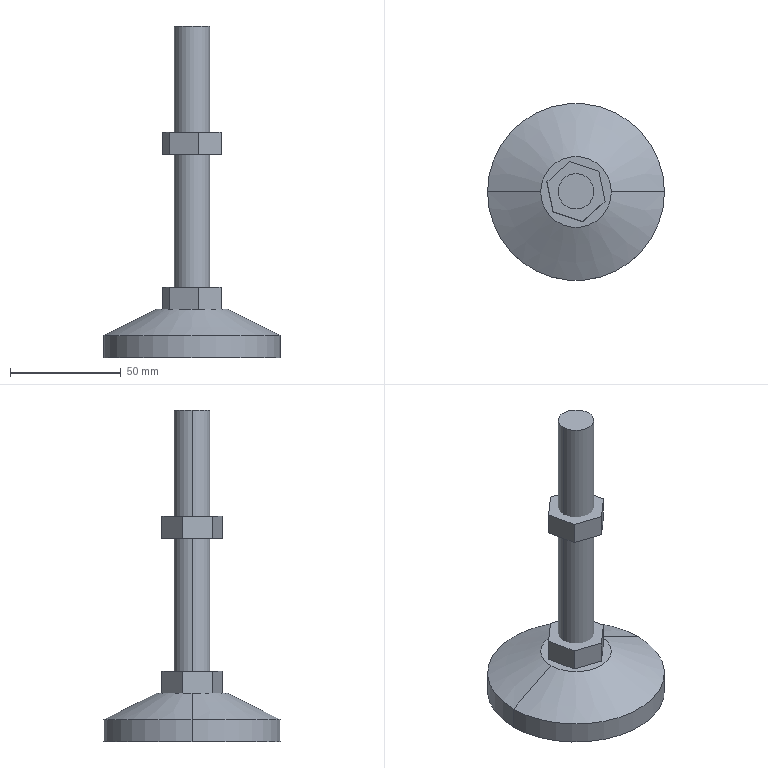Part | SolidWorks | features BaseBody 3 | 3 solids | 37 faces | box 80 x 80 x 150 mm | volume 92663 mm3 | plane 27 | cylinder 6 | torus 2 | cone 2 | commonest cylinder face diameters 16 x2 30 x2 80 x2
STEP:
#1=CARTESIAN_POINT('',(8.,0.,150.));
#2=VERTEX_POINT('',#1);
#3=CARTESIAN_POINT('',(-8.,0.,150.));
#4=VERTEX_POINT('',#3);
#5=CARTESIAN_POINT('',(0.,0.,150.));
#6=DIRECTION('',(0.,0.,1.));
#7=DIRECTION('',(1.,0.,0.));
#8=AXIS2_PLACEMENT_3D('',#5,#6,#7);
#9=CIRCLE('',#8,8.);
#10=EDGE_CURVE('',#2,#4,#9,.T.);
#11=ORIENTED_EDGE('',*,*,#10,.F.);
#12=CARTESIAN_POINT('',(8.,0.,22.));
#13=VERTEX_POINT('',#12);
#14=CARTESIAN_POINT('',(8.,0.,150.));
#15=DIRECTION('',(0.,0.,-1.));
#16=VECTOR('',#15,1000.);
#17=LINE('',#14,#16);
#18=EDGE_CURVE('',#2,#13,#17,.T.);
#19=ORIENTED_EDGE('',*,*,#18,.T.);
#20=CARTESIAN_POINT('',(-8.,0.,22.));
#21=VERTEX_POINT('',#20);
#22=CARTESIAN_POINT('',(0.,0.,22.));
#23=DIRECTION('',(0.,0.,1.));
#24=DIRECTION('',(-1.,0.,0.));
#25=AXIS2_PLACEMENT_3D('',#22,#23,#24);
#26=CIRCLE('',#25,8.);
#27=EDGE_CURVE('',#13,#21,#26,.T.);
#28=ORIENTED_EDGE('',*,*,#27,.T.);
#29=CARTESIAN_POINT('',(-8.,0.,150.));
#30=DIRECTION('',(0.,0.,-1.));
#31=VECTOR('',#30,1000.);
#32=LINE('',#29,#31);
#33=EDGE_CURVE('',#4,#21,#32,.T.);
#34=ORIENTED_EDGE('',*,*,#33,.F.);
#35=EDGE_LOOP('',(#11,#19,#28,#34));
#36=FACE_OUTER_BOUND('',#35,.T.);
#37=CARTESIAN_POINT('',(0.,0.,150.));
#38=DIRECTION('',(0.,0.,-1.));
#39=DIRECTION('',(-1.,0.,0.));
#40=AXIS2_PLACEMENT_3D('',#37,#38,#39);
#41=CYLINDRICAL_SURFACE('',#40,8.);
#42=ADVANCED_FACE('',(#36),#41,.T.);
#43=CARTESIAN_POINT('',(0.,-15.,13.));
#44=VERTEX_POINT('',#43);
#45=CARTESIAN_POINT('',(0.,15.,13.));
#46=VERTEX_POINT('',#45);
#47=CARTESIAN_POINT('',(0.,0.,13.));
#48=DIRECTION('',(0.,0.,-1.));
#49=DIRECTION('',(0.,1.,0.));
#50=AXIS2_PLACEMENT_3D('',#47,#48,#49);
#51=CIRCLE('',#50,15.);
#52=EDGE_CURVE('',#44,#46,#51,.T.);
#53=ORIENTED_EDGE('',*,*,#52,.F.);
#54=CARTESIAN_POINT('',(0.,-15.,12.));
#55=VERTEX_POINT('',#54);
#56=CARTESIAN_POINT('',(0.,-15.,13.));
#57=DIRECTION('',(0.,0.,-1.));
#58=VECTOR('',#57,1000.);
#59=LINE('',#56,#58);
#60=EDGE_CURVE('',#44,#55,#59,.T.);
#61=ORIENTED_EDGE('',*,*,#60,.T.);
#62=CARTESIAN_POINT('',(0.,15.,12.));
#63=VERTEX_POINT('',#62);
#64=CARTESIAN_POINT('',(0.,0.,12.));
#65=DIRECTION('',(0.,0.,-1.));
#66=DIRECTION('',(0.,1.,0.));
#67=AXIS2_PLACEMENT_3D('',#64,#65,#66);
#68=CIRCLE('',#67,15.);
#69=EDGE_CURVE('',#55,#63,#68,.T.);
#70=ORIENTED_EDGE('',*,*,#69,.T.);
#71=CARTESIAN_POINT('',(0.,15.,13.));
#72=DIRECTION('',(0.,0.,-1.));
#73=VECTOR('',#72,1000.);
#74=LINE('',#71,#73);
#75=EDGE_CURVE('',#46,#63,#74,.T.);
#76=ORIENTED_EDGE('',*,*,#75,.F.);
#77=EDGE_LOOP('',(#53,#61,#70,#76));
#78=FACE_OUTER_BOUND('',#77,.T.);
#79=CARTESIAN_POINT('',(0.,0.,13.));
#80=DIRECTION('',(0.,0.,-1.));
#81=DIRECTION('',(0.,1.,0.));
#82=AXIS2_PLACEMENT_3D('',#79,#80,#81);
#83=CYLINDRICAL_SURFACE('',#82,15.);
#84=ADVANCED_FACE('',(#78),#83,.F.);
#85=ORIENTED_EDGE('',*,*,#69,.F.);
#86=CARTESIAN_POINT('',(0.,-34.,0.));
#87=VERTEX_POINT('',#86);
#88=CARTESIAN_POINT('',(0.,-9.731,-17.385));
#89=DIRECTION('',(1.,0.,0.));
#90=DIRECTION('',(0.,1.,0.));
#91=AXIS2_PLACEMENT_3D('',#88,#89,#90);
#92=CIRCLE('',#91,29.854);
#93=EDGE_CURVE('',#55,#87,#92,.T.);
#94=ORIENTED_EDGE('',*,*,#93,.T.);
#95=CARTESIAN_POINT('',(0.,34.,0.));
#96=VERTEX_POINT('',#95);
#97=CARTESIAN_POINT('',(0.,0.,0.));
#98=DIRECTION('',(0.,0.,-1.));
#99=DIRECTION('',(0.,1.,0.));
#100=AXIS2_PLACEMENT_3D('',#97,#98,#99);
#101=CIRCLE('',#100,34.);
#102=EDGE_CURVE('',#87,#96,#101,.T.);
#103=ORIENTED_EDGE('',*,*,#102,.T.);
#104=CARTESIAN_POINT('',(0.,9.731,-17.385));
#105=DIRECTION('',(-1.,0.,0.));
#106=DIRECTION('',(0.,0.,1.));
#107=AXIS2_PLACEMENT_3D('',#104,#105,#106);
#108=CIRCLE('',#107,29.854);
#109=EDGE_CURVE('',#63,#96,#108,.T.);
#110=ORIENTED_EDGE('',*,*,#109,.F.);
#111=EDGE_LOOP('',(#85,#94,#103,#110));
#112=FACE_OUTER_BOUND('',#111,.T.);
#113=CARTESIAN_POINT('',(0.,0.,-17.385));
#114=DIRECTION('',(0.,0.,-1.));
#115=DIRECTION('',(0.,1.,0.));
#116=AXIS2_PLACEMENT_3D('',#113,#114,#115);
#117=TOROIDAL_SURFACE('',#116,9.731,29.854);
#118=ADVANCED_FACE('',(#112),#117,.F.);
#119=CARTESIAN_POINT('',(-16.,0.,22.));
#120=VERTEX_POINT('',#119);
#121=CARTESIAN_POINT('',(16.,0.,22.));
#122=VERTEX_POINT('',#121);
#123=CARTESIAN_POINT('',(0.,0.,22.));
#124=DIRECTION('',(0.,0.,-1.));
#125=DIRECTION('',(-1.,0.,0.));
#126=AXIS2_PLACEMENT_3D('',#123,#124,#125);
#127=CIRCLE('',#126,16.);
#128=EDGE_CURVE('',#120,#122,#127,.T.);
#129=ORIENTED_EDGE('',*,*,#128,.T.);
#130=CARTESIAN_POINT('',(40.,0.,10.));
#131=VERTEX_POINT('',#130);
#132=CARTESIAN_POINT('',(16.,0.,22.));
#133=DIRECTION('',(0.8944,0.,-0.4472));
#134=VECTOR('',#133,1000.);
#135=LINE('',#132,#134);
#136=EDGE_CURVE('',#122,#131,#135,.T.);
#137=ORIENTED_EDGE('',*,*,#136,.T.);
#138=CARTESIAN_POINT('',(-40.,0.,10.));
#139=VERTEX_POINT('',#138);
#140=CARTESIAN_POINT('',(0.,0.,10.));
#141=DIRECTION('',(0.,0.,1.));
#142=DIRECTION('',(1.,0.,0.));
#143=AXIS2_PLACEMENT_3D('',#140,#141,#142);
#144=CIRCLE('',#143,40.);
#145=EDGE_CURVE('',#131,#139,#144,.T.);
#146=ORIENTED_EDGE('',*,*,#145,.T.);
#147=CARTESIAN_POINT('',(-16.,0.,22.));
#148=DIRECTION('',(-0.8944,0.,-0.4472));
#149=VECTOR('',#148,1000.);
#150=LINE('',#147,#149);
#151=EDGE_CURVE('',#120,#139,#150,.T.);
#152=ORIENTED_EDGE('',*,*,#151,.F.);
#153=EDGE_LOOP('',(#129,#137,#146,#152));
#154=FACE_OUTER_BOUND('',#153,.T.);
#155=CARTESIAN_POINT('',(0.,0.,22.));
#156=DIRECTION('',(0.,0.,-1.));
#157=DIRECTION('',(-1.,0.,0.));
#158=AXIS2_PLACEMENT_3D('',#155,#156,#157);
#159=CONICAL_SURFACE('',#158,16.,1.107);
#160=ADVANCED_FACE('',(#154),#159,.T.);
#161=ORIENTED_EDGE('',*,*,#145,.F.);
#162=CARTESIAN_POINT('',(40.,0.,0.));
#163=VERTEX_POINT('',#162);
#164=CARTESIAN_POINT('',(40.,0.,10.));
#165=DIRECTION('',(0.,0.,-1.));
#166=VECTOR('',#165,1000.);
#167=LINE('',#164,#166);
#168=EDGE_CURVE('',#131,#163,#167,.T.);
#169=ORIENTED_EDGE('',*,*,#168,.T.);
#170=CARTESIAN_POINT('',(-40.,0.,0.));
#171=VERTEX_POINT('',#170);
#172=CARTESIAN_POINT('',(0.,0.,0.));
#173=DIRECTION('',(0.,0.,1.));
#174=DIRECTION('',(1.,0.,0.));
#175=AXIS2_PLACEMENT_3D('',#172,#173,#174);
#176=CIRCLE('',#175,40.);
#177=EDGE_CURVE('',#163,#171,#176,.T.);
#178=ORIENTED_EDGE('',*,*,#177,.T.);
#179=CARTESIAN_POINT('',(-40.,0.,10.));
#180=DIRECTION('',(0.,0.,-1.));
#181=VECTOR('',#180,1000.);
#182=LINE('',#179,#181);
#183=EDGE_CURVE('',#139,#171,#182,.T.);
#184=ORIENTED_EDGE('',*,*,#183,.F.);
#185=EDGE_LOOP('',(#161,#169,#178,#184));
#186=FACE_OUTER_BOUND('',#185,.T.);
#187=CARTESIAN_POINT('',(0.,0.,10.));
#188=DIRECTION('',(0.,0.,-1.));
#189=DIRECTION('',(-1.,0.,0.));
#190=AXIS2_PLACEMENT_3D('',#187,#188,#189);
#191=CYLINDRICAL_SURFACE('',#190,40.);
#192=ADVANCED_FACE('',(#186),#191,.T.);
#193=ORIENTED_EDGE('',*,*,#128,.F.);
#194=CARTESIAN_POINT('',(0.,0.,22.));
#195=DIRECTION('',(0.,0.,-1.));
#196=DIRECTION('',(-1.,0.,0.));
#197=AXIS2_PLACEMENT_3D('',#194,#195,#196);
#198=CIRCLE('',#197,16.);
#199=EDGE_CURVE('',#122,#120,#198,.T.);
#200=ORIENTED_EDGE('',*,*,#199,.F.);
#201=EDGE_LOOP('',(#193,#200));
#202=FACE_OUTER_BOUND('',#201,.T.);
#203=CARTESIAN_POINT('',(0.,0.,22.));
#204=DIRECTION('',(0.,0.,1.));
#205=DIRECTION('',(-1.,0.,0.));
#206=AXIS2_PLACEMENT_3D('',#203,#204,#205);
#207=CIRCLE('',#206,8.);
#208=EDGE_CURVE('',#21,#13,#207,.T.);
#209=ORIENTED_EDGE('',*,*,#208,.F.);
#210=ORIENTED_EDGE('',*,*,#27,.F.);
#211=EDGE_LOOP('',(#209,#210));
#212=FACE_BOUND('',#211,.T.);
#213=CARTESIAN_POINT('',(0.,0.,22.));
#214=DIRECTION('',(0.,0.,-1.));
#215=DIRECTION('',(-1.,0.,0.));
#216=AXIS2_PLACEMENT_3D('',#213,#214,#215);
#217=PLANE('',#216);
#218=ADVANCED_FACE('',(#202,#212),#217,.F.);
#219=CARTESIAN_POINT('',(0.,0.,13.));
#220=DIRECTION('',(0.,0.,-1.));
#221=DIRECTION('',(0.,1.,0.));
#222=AXIS2_PLACEMENT_3D('',#219,#220,#221);
#223=CIRCLE('',#222,15.);
#224=EDGE_CURVE('',#46,#44,#223,.T.);
#225=ORIENTED_EDGE('',*,*,#224,.T.);
#226=ORIENTED_EDGE('',*,*,#52,.T.);
#227=EDGE_LOOP('',(#225,#226));
#228=FACE_OUTER_BOUND('',#227,.T.);
#229=CARTESIAN_POINT('',(-11.89,7.115,13.));
#230=VERTEX_POINT('',#229);
#231=CARTESIAN_POINT('',(0.2164,13.855,13.));
#232=VERTEX_POINT('',#231);
#233=CARTESIAN_POINT('',(-11.89,7.115,13.));
#234=DIRECTION('',(0.8737,0.4864,0.));
#235=VECTOR('',#234,1000.);
#236=LINE('',#233,#235);
#237=EDGE_CURVE('',#230,#232,#236,.T.);
#238=ORIENTED_EDGE('',*,*,#237,.F.);
#239=CARTESIAN_POINT('',(-12.107,-6.74,13.));
#240=VERTEX_POINT('',#239);
#241=CARTESIAN_POINT('',(-12.107,-6.74,13.));
#242=DIRECTION('',(0.01561,0.9999,0.));
#243=VECTOR('',#242,1000.);
#244=LINE('',#241,#243);
#245=EDGE_CURVE('',#240,#230,#244,.T.);
#246=ORIENTED_EDGE('',*,*,#245,.F.);
#247=CARTESIAN_POINT('',(-0.2164,-13.855,13.));
#248=VERTEX_POINT('',#247);
#249=CARTESIAN_POINT('',(-0.2164,-13.855,13.));
#250=DIRECTION('',(-0.8581,0.5135,0.));
#251=VECTOR('',#250,1000.);
#252=LINE('',#249,#251);
#253=EDGE_CURVE('',#248,#240,#252,.T.);
#254=ORIENTED_EDGE('',*,*,#253,.F.);
#255=CARTESIAN_POINT('',(11.89,-7.115,13.));
#256=VERTEX_POINT('',#255);
#257=CARTESIAN_POINT('',(11.89,-7.115,13.));
#258=DIRECTION('',(-0.8737,-0.4864,0.));
#259=VECTOR('',#258,1000.);
#260=LINE('',#257,#259);
#261=EDGE_CURVE('',#256,#248,#260,.T.);
#262=ORIENTED_EDGE('',*,*,#261,.F.);
#263=CARTESIAN_POINT('',(12.107,6.74,13.));
#264=VERTEX_POINT('',#263);
#265=CARTESIAN_POINT('',(12.107,6.74,13.));
#266=DIRECTION('',(-0.01561,-0.9999,0.));
#267=VECTOR('',#266,1000.);
#268=LINE('',#265,#267);
#269=EDGE_CURVE('',#264,#256,#268,.T.);
#270=ORIENTED_EDGE('',*,*,#269,.F.);
#271=CARTESIAN_POINT('',(0.2164,13.855,13.));
#272=DIRECTION('',(0.8581,-0.5135,0.));
#273=VECTOR('',#272,1000.);
#274=LINE('',#271,#273);
#275=EDGE_CURVE('',#232,#264,#274,.T.);
#276=ORIENTED_EDGE('',*,*,#275,.F.);
#277=EDGE_LOOP('',(#238,#246,#254,#262,#270,#276));
#278=FACE_BOUND('',#277,.T.);
#279=CARTESIAN_POINT('',(0.,0.,13.));
#280=DIRECTION('',(0.,0.,-1.));
#281=DIRECTION('',(0.,1.,0.));
#282=AXIS2_PLACEMENT_3D('',#279,#280,#281);
#283=PLANE('',#282);
#284=ADVANCED_FACE('',(#228,#278),#283,.T.);
#285=ORIENTED_EDGE('',*,*,#168,.F.);
#286=CARTESIAN_POINT('',(0.,0.,10.));
#287=DIRECTION('',(0.,0.,1.));
#288=DIRECTION('',(1.,0.,0.));
#289=AXIS2_PLACEMENT_3D('',#286,#287,#288);
#290=CIRCLE('',#289,40.);
#291=EDGE_CURVE('',#139,#131,#290,.T.);
#292=ORIENTED_EDGE('',*,*,#291,.F.);
#293=ORIENTED_EDGE('',*,*,#183,.T.);
#294=CARTESIAN_POINT('',(0.,0.,0.));
#295=DIRECTION('',(0.,0.,1.));
#296=DIRECTION('',(1.,0.,0.));
#297=AXIS2_PLACEMENT_3D('',#294,#295,#296);
#298=CIRCLE('',#297,40.);
#299=EDGE_CURVE('',#171,#163,#298,.T.);
#300=ORIENTED_EDGE('',*,*,#299,.T.);
#301=EDGE_LOOP('',(#285,#292,#293,#300));
#302=FACE_OUTER_BOUND('',#301,.T.);
#303=CARTESIAN_POINT('',(0.,0.,10.));
#304=DIRECTION('',(0.,0.,-1.));
#305=DIRECTION('',(-1.,0.,0.));
#306=AXIS2_PLACEMENT_3D('',#303,#304,#305);
#307=CYLINDRICAL_SURFACE('',#306,40.);
#308=ADVANCED_FACE('',(#302),#307,.T.);
#309=CARTESIAN_POINT('',(0.,0.,0.));
#310=DIRECTION('',(0.,0.,-1.));
#311=DIRECTION('',(0.,1.,0.));
#312=AXIS2_PLACEMENT_3D('',#309,#310,#311);
#313=CIRCLE('',#312,34.);
#314=EDGE_CURVE('',#96,#87,#313,.T.);
#315=ORIENTED_EDGE('',*,*,#314,.F.);
#316=ORIENTED_EDGE('',*,*,#102,.F.);
#317=EDGE_LOOP('',(#315,#316));
#318=FACE_BOUND('',#317,.T.);
#319=ORIENTED_EDGE('',*,*,#299,.F.);
#320=ORIENTED_EDGE('',*,*,#177,.F.);
#321=EDGE_LOOP('',(#319,#320));
#322=FACE_OUTER_BOUND('',#321,.T.);
#323=CARTESIAN_POINT('',(0.,0.,0.));
#324=DIRECTION('',(0.,0.,1.));
#325=DIRECTION('',(1.,0.,0.));
#326=AXIS2_PLACEMENT_3D('',#323,#324,#325);
#327=PLANE('',#326);
#328=ADVANCED_FACE('',(#318,#322),#327,.F.);
#329=ORIENTED_EDGE('',*,*,#136,.F.);
#330=ORIENTED_EDGE('',*,*,#199,.T.);
#331=ORIENTED_EDGE('',*,*,#151,.T.);
#332=ORIENTED_EDGE('',*,*,#291,.T.);
#333=EDGE_LOOP('',(#329,#330,#331,#332));
#334=FACE_OUTER_BOUND('',#333,.T.);
#335=CARTESIAN_POINT('',(0.,0.,22.));
#336=DIRECTION('',(0.,0.,-1.));
#337=DIRECTION('',(-1.,0.,0.));
#338=AXIS2_PLACEMENT_3D('',#335,#336,#337);
#339=CONICAL_SURFACE('',#338,16.,1.107);
#340=ADVANCED_FACE('',(#334),#339,.T.);
#341=ORIENTED_EDGE('',*,*,#93,.F.);
#342=CARTESIAN_POINT('',(0.,0.,12.));
#343=DIRECTION('',(0.,0.,-1.));
#344=DIRECTION('',(0.,1.,0.));
#345=AXIS2_PLACEMENT_3D('',#342,#343,#344);
#346=CIRCLE('',#345,15.);
#347=EDGE_CURVE('',#63,#55,#346,.T.);
#348=ORIENTED_EDGE('',*,*,#347,.F.);
#349=ORIENTED_EDGE('',*,*,#109,.T.);
#350=ORIENTED_EDGE('',*,*,#314,.T.);
#351=EDGE_LOOP('',(#341,#348,#349,#350));
#352=FACE_OUTER_BOUND('',#351,.T.);
#353=CARTESIAN_POINT('',(0.,0.,-17.385));
#354=DIRECTION('',(0.,0.,-1.));
#355=DIRECTION('',(0.,1.,0.));
#356=AXIS2_PLACEMENT_3D('',#353,#354,#355);
#357=TOROIDAL_SURFACE('',#356,9.731,29.854);
#358=ADVANCED_FACE('',(#352),#357,.F.);
#359=ORIENTED_EDGE('',*,*,#60,.F.);
#360=ORIENTED_EDGE('',*,*,#224,.F.);
#361=ORIENTED_EDGE('',*,*,#75,.T.);
#362=ORIENTED_EDGE('',*,*,#347,.T.);
#363=EDGE_LOOP('',(#359,#360,#361,#362));
#364=FACE_OUTER_BOUND('',#363,.T.);
#365=CARTESIAN_POINT('',(0.,0.,13.));
#366=DIRECTION('',(0.,0.,-1.));
#367=DIRECTION('',(0.,1.,0.));
#368=AXIS2_PLACEMENT_3D('',#365,#366,#367);
#369=CYLINDRICAL_SURFACE('',#368,15.);
#370=ADVANCED_FACE('',(#364),#369,.F.);
#371=ORIENTED_EDGE('',*,*,#245,.T.);
#372=CARTESIAN_POINT('',(-11.89,7.115,3.));
#373=VERTEX_POINT('',#372);
#374=CARTESIAN_POINT('',(-11.89,7.115,3.));
#375=DIRECTION('',(0.,0.,1.));
#376=VECTOR('',#375,1000.);
#377=LINE('',#374,#376);
#378=EDGE_CURVE('',#373,#230,#377,.T.);
#379=ORIENTED_EDGE('',*,*,#378,.F.);
#380=CARTESIAN_POINT('',(-12.107,-6.74,3.));
#381=VERTEX_POINT('',#380);
#382=CARTESIAN_POINT('',(-12.107,-6.74,3.));
#383=DIRECTION('',(0.01561,0.9999,0.));
#384=VECTOR('',#383,1000.);
#385=LINE('',#382,#384);
#386=EDGE_CURVE('',#381,#373,#385,.T.);
#387=ORIENTED_EDGE('',*,*,#386,.F.);
#388=CARTESIAN_POINT('',(-12.107,-6.74,3.));
#389=DIRECTION('',(0.,0.,1.));
#390=VECTOR('',#389,1000.);
#391=LINE('',#388,#390);
#392=EDGE_CURVE('',#381,#240,#391,.T.);
#393=ORIENTED_EDGE('',*,*,#392,.T.);
#394=EDGE_LOOP('',(#371,#379,#387,#393));
#395=FACE_OUTER_BOUND('',#394,.T.);
#396=CARTESIAN_POINT('',(-12.107,-6.74,3.));
#397=DIRECTION('',(0.9999,-0.01561,0.));
#398=DIRECTION('',(0.01561,0.9999,0.));
#399=AXIS2_PLACEMENT_3D('',#396,#397,#398);
#400=PLANE('',#399);
#401=ADVANCED_FACE('',(#395),#400,.F.);
#402=ORIENTED_EDGE('',*,*,#237,.T.);
#403=CARTESIAN_POINT('',(0.2164,13.855,3.));
#404=VERTEX_POINT('',#403);
#405=CARTESIAN_POINT('',(0.2164,13.855,3.));
#406=DIRECTION('',(0.,0.,1.));
#407=VECTOR('',#406,1000.);
#408=LINE('',#405,#407);
#409=EDGE_CURVE('',#404,#232,#408,.T.);
#410=ORIENTED_EDGE('',*,*,#409,.F.);
#411=CARTESIAN_POINT('',(-11.89,7.115,3.));
#412=DIRECTION('',(0.8737,0.4864,0.));
#413=VECTOR('',#412,1000.);
#414=LINE('',#411,#413);
#415=EDGE_CURVE('',#373,#404,#414,.T.);
#416=ORIENTED_EDGE('',*,*,#415,.F.);
#417=ORIENTED_EDGE('',*,*,#378,.T.);
#418=EDGE_LOOP('',(#402,#410,#416,#417));
#419=FACE_OUTER_BOUND('',#418,.T.);
#420=CARTESIAN_POINT('',(-11.89,7.115,3.));
#421=DIRECTION('',(0.4864,-0.8737,0.));
#422=DIRECTION('',(0.8737,0.4864,0.));
#423=AXIS2_PLACEMENT_3D('',#420,#421,#422);
#424=PLANE('',#423);
#425=ADVANCED_FACE('',(#419),#424,.F.);
#426=ORIENTED_EDGE('',*,*,#275,.T.);
#427=CARTESIAN_POINT('',(12.107,6.74,3.));
#428=VERTEX_POINT('',#427);
#429=CARTESIAN_POINT('',(12.107,6.74,3.));
#430=DIRECTION('',(0.,0.,1.));
#431=VECTOR('',#430,1000.);
#432=LINE('',#429,#431);
#433=EDGE_CURVE('',#428,#264,#432,.T.);
#434=ORIENTED_EDGE('',*,*,#433,.F.);
#435=CARTESIAN_POINT('',(0.2164,13.855,3.));
#436=DIRECTION('',(0.8581,-0.5135,0.));
#437=VECTOR('',#436,1000.);
#438=LINE('',#435,#437);
#439=EDGE_CURVE('',#404,#428,#438,.T.);
#440=ORIENTED_EDGE('',*,*,#439,.F.);
#441=ORIENTED_EDGE('',*,*,#409,.T.);
#442=EDGE_LOOP('',(#426,#434,#440,#441));
#443=FACE_OUTER_BOUND('',#442,.T.);
#444=CARTESIAN_POINT('',(0.2164,13.855,3.));
#445=DIRECTION('',(-0.5135,-0.8581,0.));
#446=DIRECTION('',(0.8581,-0.5135,0.));
#447=AXIS2_PLACEMENT_3D('',#444,#445,#446);
#448=PLANE('',#447);
#449=ADVANCED_FACE('',(#443),#448,.F.);
#450=ORIENTED_EDGE('',*,*,#269,.T.);
#451=CARTESIAN_POINT('',(11.89,-7.115,3.));
#452=VERTEX_POINT('',#451);
#453=CARTESIAN_POINT('',(11.89,-7.115,3.));
#454=DIRECTION('',(0.,0.,1.));
#455=VECTOR('',#454,1000.);
#456=LINE('',#453,#455);
#457=EDGE_CURVE('',#452,#256,#456,.T.);
#458=ORIENTED_EDGE('',*,*,#457,.F.);
#459=CARTESIAN_POINT('',(12.107,6.74,3.));
#460=DIRECTION('',(-0.01561,-0.9999,0.));
#461=VECTOR('',#460,1000.);
#462=LINE('',#459,#461);
#463=EDGE_CURVE('',#428,#452,#462,.T.);
#464=ORIENTED_EDGE('',*,*,#463,.F.);
#465=ORIENTED_EDGE('',*,*,#433,.T.);
#466=EDGE_LOOP('',(#450,#458,#464,#465));
#467=FACE_OUTER_BOUND('',#466,.T.);
#468=CARTESIAN_POINT('',(12.107,6.74,3.));
#469=DIRECTION('',(-0.9999,0.01561,0.));
#470=DIRECTION('',(-0.01561,-0.9999,0.));
#471=AXIS2_PLACEMENT_3D('',#468,#469,#470);
#472=PLANE('',#471);
#473=ADVANCED_FACE('',(#467),#472,.F.);
#474=ORIENTED_EDGE('',*,*,#261,.T.);
#475=CARTESIAN_POINT('',(-0.2164,-13.855,3.));
#476=VERTEX_POINT('',#475);
#477=CARTESIAN_POINT('',(-0.2164,-13.855,3.));
#478=DIRECTION('',(0.,0.,1.));
#479=VECTOR('',#478,1000.);
#480=LINE('',#477,#479);
#481=EDGE_CURVE('',#476,#248,#480,.T.);
#482=ORIENTED_EDGE('',*,*,#481,.F.);
#483=CARTESIAN_POINT('',(11.89,-7.115,3.));
#484=DIRECTION('',(-0.8737,-0.4864,0.));
#485=VECTOR('',#484,1000.);
#486=LINE('',#483,#485);
#487=EDGE_CURVE('',#452,#476,#486,.T.);
#488=ORIENTED_EDGE('',*,*,#487,.F.);
#489=ORIENTED_EDGE('',*,*,#457,.T.);
#490=EDGE_LOOP('',(#474,#482,#488,#489));
#491=FACE_OUTER_BOUND('',#490,.T.);
#492=CARTESIAN_POINT('',(11.89,-7.115,3.));
#493=DIRECTION('',(-0.4864,0.8737,0.));
#494=DIRECTION('',(-0.8737,-0.4864,0.));
#495=AXIS2_PLACEMENT_3D('',#492,#493,#494);
#496=PLANE('',#495);
#497=ADVANCED_FACE('',(#491),#496,.F.);
#498=ORIENTED_EDGE('',*,*,#253,.T.);
#499=ORIENTED_EDGE('',*,*,#392,.F.);
#500=CARTESIAN_POINT('',(-0.2164,-13.855,3.));
#501=DIRECTION('',(-0.8581,0.5135,0.));
#502=VECTOR('',#501,1000.);
#503=LINE('',#500,#502);
#504=EDGE_CURVE('',#476,#381,#503,.T.);
#505=ORIENTED_EDGE('',*,*,#504,.F.);
#506=ORIENTED_EDGE('',*,*,#481,.T.);
#507=EDGE_LOOP('',(#498,#499,#505,#506));
#508=FACE_OUTER_BOUND('',#507,.T.);
#509=CARTESIAN_POINT('',(-0.2164,-13.855,3.));
#510=DIRECTION('',(0.5135,0.8581,0.));
#511=DIRECTION('',(-0.8581,0.5135,0.));
#512=AXIS2_PLACEMENT_3D('',#509,#510,#511);
#513=PLANE('',#512);
#514=ADVANCED_FACE('',(#508),#513,.F.);
#515=ORIENTED_EDGE('',*,*,#386,.T.);
#516=ORIENTED_EDGE('',*,*,#415,.T.);
#517=ORIENTED_EDGE('',*,*,#439,.T.);
#518=ORIENTED_EDGE('',*,*,#463,.T.);
#519=ORIENTED_EDGE('',*,*,#487,.T.);
#520=ORIENTED_EDGE('',*,*,#504,.T.);
#521=EDGE_LOOP('',(#515,#516,#517,#518,#519,#520));
#522=FACE_OUTER_BOUND('',#521,.T.);
#523=CARTESIAN_POINT('',(-11.89,7.115,3.));
#524=DIRECTION('',(0.,0.,-1.));
#525=DIRECTION('',(0.,1.,0.));
#526=AXIS2_PLACEMENT_3D('',#523,#524,#525);
#527=PLANE('',#526);
#528=ADVANCED_FACE('',(#522),#527,.T.);
#529=ORIENTED_EDGE('',*,*,#18,.F.);
#530=CARTESIAN_POINT('',(0.,0.,150.));
#531=DIRECTION('',(0.,0.,1.));
#532=DIRECTION('',(1.,0.,0.));
#533=AXIS2_PLACEMENT_3D('',#530,#531,#532);
#534=CIRCLE('',#533,8.);
#535=EDGE_CURVE('',#4,#2,#534,.T.);
#536=ORIENTED_EDGE('',*,*,#535,.F.);
#537=ORIENTED_EDGE('',*,*,#33,.T.);
#538=ORIENTED_EDGE('',*,*,#208,.T.);
#539=EDGE_LOOP('',(#529,#536,#537,#538));
#540=FACE_OUTER_BOUND('',#539,.T.);
#541=CARTESIAN_POINT('',(0.,0.,150.));
#542=DIRECTION('',(0.,0.,-1.));
#543=DIRECTION('',(-1.,0.,0.));
#544=AXIS2_PLACEMENT_3D('',#541,#542,#543);
#545=CYLINDRICAL_SURFACE('',#544,8.);
#546=ADVANCED_FACE('',(#540),#545,.T.);
#547=ORIENTED_EDGE('',*,*,#535,.T.);
#548=ORIENTED_EDGE('',*,*,#10,.T.);
#549=EDGE_LOOP('',(#547,#548));
#550=FACE_OUTER_BOUND('',#549,.T.);
#551=CARTESIAN_POINT('',(0.,0.,150.));
#552=DIRECTION('',(0.,0.,1.));
#553=DIRECTION('',(1.,0.,0.));
#554=AXIS2_PLACEMENT_3D('',#551,#552,#553);
#555=PLANE('',#554);
#556=ADVANCED_FACE('',(#550),#555,.T.);
#557=CLOSED_SHELL('',(#42,#84,#118,#160,#192,#218,#284,#308,#328,#340,#358,#370,#401,#425,#449,#473,#497,#514,#528,#546,#556));
#558=MANIFOLD_SOLID_BREP('',#557);
#559=CARTESIAN_POINT('',(13.138,-4.403,22.));
#560=VERTEX_POINT('',#559);
#561=CARTESIAN_POINT('',(10.382,9.177,22.));
#562=VERTEX_POINT('',#561);
#563=CARTESIAN_POINT('',(13.138,-4.403,22.));
#564=DIRECTION('',(-0.1989,0.98,0.));
#565=VECTOR('',#564,1000.);
#566=LINE('',#563,#565);
#567=EDGE_CURVE('',#560,#562,#566,.T.);
#568=ORIENTED_EDGE('',*,*,#567,.T.);
#569=CARTESIAN_POINT('',(10.382,9.177,32.));
#570=VERTEX_POINT('',#569);
#571=CARTESIAN_POINT('',(10.382,9.177,32.));
#572=DIRECTION('',(0.,0.,-1.));
#573=VECTOR('',#572,1000.);
#574=LINE('',#571,#573);
#575=EDGE_CURVE('',#570,#562,#574,.T.);
#576=ORIENTED_EDGE('',*,*,#575,.F.);
#577=CARTESIAN_POINT('',(13.138,-4.403,32.));
#578=VERTEX_POINT('',#577);
#579=CARTESIAN_POINT('',(13.138,-4.403,32.));
#580=DIRECTION('',(-0.1989,0.98,0.));
#581=VECTOR('',#580,1000.);
#582=LINE('',#579,#581);
#583=EDGE_CURVE('',#578,#570,#582,.T.);
#584=ORIENTED_EDGE('',*,*,#583,.F.);
#585=CARTESIAN_POINT('',(13.138,-4.403,32.));
#586=DIRECTION('',(0.,0.,-1.));
#587=VECTOR('',#586,1000.);
#588=LINE('',#585,#587);
#589=EDGE_CURVE('',#578,#560,#588,.T.);
#590=ORIENTED_EDGE('',*,*,#589,.T.);
#591=EDGE_LOOP('',(#568,#576,#584,#590));
#592=FACE_OUTER_BOUND('',#591,.T.);
#593=CARTESIAN_POINT('',(13.138,-4.403,32.));
#594=DIRECTION('',(-0.98,-0.1989,0.));
#595=DIRECTION('',(0.1989,-0.98,0.));
#596=AXIS2_PLACEMENT_3D('',#593,#594,#595);
#597=PLANE('',#596);
#598=ADVANCED_FACE('',(#592),#597,.F.);
#599=CARTESIAN_POINT('',(-2.756,13.579,22.));
#600=VERTEX_POINT('',#599);
#601=CARTESIAN_POINT('',(10.382,9.177,22.));
#602=DIRECTION('',(-0.9482,0.3177,0.));
#603=VECTOR('',#602,1000.);
#604=LINE('',#601,#603);
#605=EDGE_CURVE('',#562,#600,#604,.T.);
#606=ORIENTED_EDGE('',*,*,#605,.T.);
#607=CARTESIAN_POINT('',(-2.756,13.579,32.));
#608=VERTEX_POINT('',#607);
#609=CARTESIAN_POINT('',(-2.756,13.579,32.));
#610=DIRECTION('',(0.,0.,-1.));
#611=VECTOR('',#610,1000.);
#612=LINE('',#609,#611);
#613=EDGE_CURVE('',#608,#600,#612,.T.);
#614=ORIENTED_EDGE('',*,*,#613,.F.);
#615=CARTESIAN_POINT('',(10.382,9.177,32.));
#616=DIRECTION('',(-0.9482,0.3177,0.));
#617=VECTOR('',#616,1000.);
#618=LINE('',#615,#617);
#619=EDGE_CURVE('',#570,#608,#618,.T.);
#620=ORIENTED_EDGE('',*,*,#619,.F.);
#621=ORIENTED_EDGE('',*,*,#575,.T.);
#622=EDGE_LOOP('',(#606,#614,#620,#621));
#623=FACE_OUTER_BOUND('',#622,.T.);
#624=CARTESIAN_POINT('',(10.382,9.177,32.));
#625=DIRECTION('',(-0.3177,-0.9482,0.));
#626=DIRECTION('',(0.9482,-0.3177,0.));
#627=AXIS2_PLACEMENT_3D('',#624,#625,#626);
#628=PLANE('',#627);
#629=ADVANCED_FACE('',(#623),#628,.F.);
#630=CARTESIAN_POINT('',(-13.138,4.403,22.));
#631=VERTEX_POINT('',#630);
#632=CARTESIAN_POINT('',(-2.756,13.579,22.));
#633=DIRECTION('',(-0.7493,-0.6623,0.));
#634=VECTOR('',#633,1000.);
#635=LINE('',#632,#634);
#636=EDGE_CURVE('',#600,#631,#635,.T.);
#637=ORIENTED_EDGE('',*,*,#636,.T.);
#638=CARTESIAN_POINT('',(-13.138,4.403,32.));
#639=VERTEX_POINT('',#638);
#640=CARTESIAN_POINT('',(-13.138,4.403,32.));
#641=DIRECTION('',(0.,0.,-1.));
#642=VECTOR('',#641,1000.);
#643=LINE('',#640,#642);
#644=EDGE_CURVE('',#639,#631,#643,.T.);
#645=ORIENTED_EDGE('',*,*,#644,.F.);
#646=CARTESIAN_POINT('',(-2.756,13.579,32.));
#647=DIRECTION('',(-0.7493,-0.6623,0.));
#648=VECTOR('',#647,1000.);
#649=LINE('',#646,#648);
#650=EDGE_CURVE('',#608,#639,#649,.T.);
#651=ORIENTED_EDGE('',*,*,#650,.F.);
#652=ORIENTED_EDGE('',*,*,#613,.T.);
#653=EDGE_LOOP('',(#637,#645,#651,#652));
#654=FACE_OUTER_BOUND('',#653,.T.);
#655=CARTESIAN_POINT('',(-2.756,13.579,32.));
#656=DIRECTION('',(0.6623,-0.7493,0.));
#657=DIRECTION('',(0.7493,0.6623,0.));
#658=AXIS2_PLACEMENT_3D('',#655,#656,#657);
#659=PLANE('',#658);
#660=ADVANCED_FACE('',(#654),#659,.F.);
#661=CARTESIAN_POINT('',(-10.382,-9.177,22.));
#662=VERTEX_POINT('',#661);
#663=CARTESIAN_POINT('',(-13.138,4.403,22.));
#664=DIRECTION('',(0.1989,-0.98,0.));
#665=VECTOR('',#664,1000.);
#666=LINE('',#663,#665);
#667=EDGE_CURVE('',#631,#662,#666,.T.);
#668=ORIENTED_EDGE('',*,*,#667,.T.);
#669=CARTESIAN_POINT('',(-10.382,-9.177,32.));
#670=VERTEX_POINT('',#669);
#671=CARTESIAN_POINT('',(-10.382,-9.177,32.));
#672=DIRECTION('',(0.,0.,-1.));
#673=VECTOR('',#672,1000.);
#674=LINE('',#671,#673);
#675=EDGE_CURVE('',#670,#662,#674,.T.);
#676=ORIENTED_EDGE('',*,*,#675,.F.);
#677=CARTESIAN_POINT('',(-13.138,4.403,32.));
#678=DIRECTION('',(0.1989,-0.98,0.));
#679=VECTOR('',#678,1000.);
#680=LINE('',#677,#679);
#681=EDGE_CURVE('',#639,#670,#680,.T.);
#682=ORIENTED_EDGE('',*,*,#681,.F.);
#683=ORIENTED_EDGE('',*,*,#644,.T.);
#684=EDGE_LOOP('',(#668,#676,#682,#683));
#685=FACE_OUTER_BOUND('',#684,.T.);
#686=CARTESIAN_POINT('',(-13.138,4.403,32.));
#687=DIRECTION('',(0.98,0.1989,0.));
#688=DIRECTION('',(-0.1989,0.98,0.));
#689=AXIS2_PLACEMENT_3D('',#686,#687,#688);
#690=PLANE('',#689);
#691=ADVANCED_FACE('',(#685),#690,.F.);
#692=CARTESIAN_POINT('',(2.756,-13.579,22.));
#693=VERTEX_POINT('',#692);
#694=CARTESIAN_POINT('',(-10.382,-9.177,22.));
#695=DIRECTION('',(0.9482,-0.3177,0.));
#696=VECTOR('',#695,1000.);
#697=LINE('',#694,#696);
#698=EDGE_CURVE('',#662,#693,#697,.T.);
#699=ORIENTED_EDGE('',*,*,#698,.T.);
#700=CARTESIAN_POINT('',(2.756,-13.579,32.));
#701=VERTEX_POINT('',#700);
#702=CARTESIAN_POINT('',(2.756,-13.579,32.));
#703=DIRECTION('',(0.,0.,-1.));
#704=VECTOR('',#703,1000.);
#705=LINE('',#702,#704);
#706=EDGE_CURVE('',#701,#693,#705,.T.);
#707=ORIENTED_EDGE('',*,*,#706,.F.);
#708=CARTESIAN_POINT('',(-10.382,-9.177,32.));
#709=DIRECTION('',(0.9482,-0.3177,0.));
#710=VECTOR('',#709,1000.);
#711=LINE('',#708,#710);
#712=EDGE_CURVE('',#670,#701,#711,.T.);
#713=ORIENTED_EDGE('',*,*,#712,.F.);
#714=ORIENTED_EDGE('',*,*,#675,.T.);
#715=EDGE_LOOP('',(#699,#707,#713,#714));
#716=FACE_OUTER_BOUND('',#715,.T.);
#717=CARTESIAN_POINT('',(-10.382,-9.177,32.));
#718=DIRECTION('',(0.3177,0.9482,0.));
#719=DIRECTION('',(-0.9482,0.3177,0.));
#720=AXIS2_PLACEMENT_3D('',#717,#718,#719);
#721=PLANE('',#720);
#722=ADVANCED_FACE('',(#716),#721,.F.);
#723=CARTESIAN_POINT('',(2.756,-13.579,22.));
#724=DIRECTION('',(0.7493,0.6623,0.));
#725=VECTOR('',#724,1000.);
#726=LINE('',#723,#725);
#727=EDGE_CURVE('',#693,#560,#726,.T.);
#728=ORIENTED_EDGE('',*,*,#727,.T.);
#729=ORIENTED_EDGE('',*,*,#589,.F.);
#730=CARTESIAN_POINT('',(2.756,-13.579,32.));
#731=DIRECTION('',(0.7493,0.6623,0.));
#732=VECTOR('',#731,1000.);
#733=LINE('',#730,#732);
#734=EDGE_CURVE('',#701,#578,#733,.T.);
#735=ORIENTED_EDGE('',*,*,#734,.F.);
#736=ORIENTED_EDGE('',*,*,#706,.T.);
#737=EDGE_LOOP('',(#728,#729,#735,#736));
#738=FACE_OUTER_BOUND('',#737,.T.);
#739=CARTESIAN_POINT('',(2.756,-13.579,32.));
#740=DIRECTION('',(-0.6623,0.7493,0.));
#741=DIRECTION('',(-0.7493,-0.6623,0.));
#742=AXIS2_PLACEMENT_3D('',#739,#740,#741);
#743=PLANE('',#742);
#744=ADVANCED_FACE('',(#738),#743,.F.);
#745=ORIENTED_EDGE('',*,*,#583,.T.);
#746=ORIENTED_EDGE('',*,*,#619,.T.);
#747=ORIENTED_EDGE('',*,*,#650,.T.);
#748=ORIENTED_EDGE('',*,*,#681,.T.);
#749=ORIENTED_EDGE('',*,*,#712,.T.);
#750=ORIENTED_EDGE('',*,*,#734,.T.);
#751=EDGE_LOOP('',(#745,#746,#747,#748,#749,#750));
#752=FACE_OUTER_BOUND('',#751,.T.);
#753=CARTESIAN_POINT('',(10.382,9.177,32.));
#754=DIRECTION('',(0.,0.,1.));
#755=DIRECTION('',(1.,0.,0.));
#756=AXIS2_PLACEMENT_3D('',#753,#754,#755);
#757=PLANE('',#756);
#758=ADVANCED_FACE('',(#752),#757,.T.);
#759=ORIENTED_EDGE('',*,*,#567,.F.);
#760=ORIENTED_EDGE('',*,*,#727,.F.);
#761=ORIENTED_EDGE('',*,*,#698,.F.);
#762=ORIENTED_EDGE('',*,*,#667,.F.);
#763=ORIENTED_EDGE('',*,*,#636,.F.);
#764=ORIENTED_EDGE('',*,*,#605,.F.);
#765=EDGE_LOOP('',(#759,#760,#761,#762,#763,#764));
#766=FACE_OUTER_BOUND('',#765,.T.);
#767=CARTESIAN_POINT('',(10.382,9.177,22.));
#768=DIRECTION('',(0.,0.,1.));
#769=DIRECTION('',(1.,0.,0.));
#770=AXIS2_PLACEMENT_3D('',#767,#768,#769);
#771=PLANE('',#770);
#772=ADVANCED_FACE('',(#766),#771,.F.);
#773=CLOSED_SHELL('',(#598,#629,#660,#691,#722,#744,#758,#772));
#774=MANIFOLD_SOLID_BREP('',#773);
#775=CARTESIAN_POINT('',(13.138,-4.403,92.));
#776=VERTEX_POINT('',#775);
#777=CARTESIAN_POINT('',(10.382,9.177,92.));
#778=VERTEX_POINT('',#777);
#779=CARTESIAN_POINT('',(13.138,-4.403,92.));
#780=DIRECTION('',(-0.1989,0.98,0.));
#781=VECTOR('',#780,1000.);
#782=LINE('',#779,#781);
#783=EDGE_CURVE('',#776,#778,#782,.T.);
#784=ORIENTED_EDGE('',*,*,#783,.T.);
#785=CARTESIAN_POINT('',(10.382,9.177,102.));
#786=VERTEX_POINT('',#785);
#787=CARTESIAN_POINT('',(10.382,9.177,102.));
#788=DIRECTION('',(0.,0.,-1.));
#789=VECTOR('',#788,1000.);
#790=LINE('',#787,#789);
#791=EDGE_CURVE('',#786,#778,#790,.T.);
#792=ORIENTED_EDGE('',*,*,#791,.F.);
#793=CARTESIAN_POINT('',(13.138,-4.403,102.));
#794=VERTEX_POINT('',#793);
#795=CARTESIAN_POINT('',(13.138,-4.403,102.));
#796=DIRECTION('',(-0.1989,0.98,0.));
#797=VECTOR('',#796,1000.);
#798=LINE('',#795,#797);
#799=EDGE_CURVE('',#794,#786,#798,.T.);
#800=ORIENTED_EDGE('',*,*,#799,.F.);
#801=CARTESIAN_POINT('',(13.138,-4.403,102.));
#802=DIRECTION('',(0.,0.,-1.));
#803=VECTOR('',#802,1000.);
#804=LINE('',#801,#803);
#805=EDGE_CURVE('',#794,#776,#804,.T.);
#806=ORIENTED_EDGE('',*,*,#805,.T.);
#807=EDGE_LOOP('',(#784,#792,#800,#806));
#808=FACE_OUTER_BOUND('',#807,.T.);
#809=CARTESIAN_POINT('',(13.138,-4.403,102.));
#810=DIRECTION('',(-0.98,-0.1989,0.));
#811=DIRECTION('',(0.1989,-0.98,0.));
#812=AXIS2_PLACEMENT_3D('',#809,#810,#811);
#813=PLANE('',#812);
#814=ADVANCED_FACE('',(#808),#813,.F.);
#815=CARTESIAN_POINT('',(-2.756,13.579,92.));
#816=VERTEX_POINT('',#815);
#817=CARTESIAN_POINT('',(10.382,9.177,92.));
#818=DIRECTION('',(-0.9482,0.3177,0.));
#819=VECTOR('',#818,1000.);
#820=LINE('',#817,#819);
#821=EDGE_CURVE('',#778,#816,#820,.T.);
#822=ORIENTED_EDGE('',*,*,#821,.T.);
#823=CARTESIAN_POINT('',(-2.756,13.579,102.));
#824=VERTEX_POINT('',#823);
#825=CARTESIAN_POINT('',(-2.756,13.579,102.));
#826=DIRECTION('',(0.,0.,-1.));
#827=VECTOR('',#826,1000.);
#828=LINE('',#825,#827);
#829=EDGE_CURVE('',#824,#816,#828,.T.);
#830=ORIENTED_EDGE('',*,*,#829,.F.);
#831=CARTESIAN_POINT('',(10.382,9.177,102.));
#832=DIRECTION('',(-0.9482,0.3177,0.));
#833=VECTOR('',#832,1000.);
#834=LINE('',#831,#833);
#835=EDGE_CURVE('',#786,#824,#834,.T.);
#836=ORIENTED_EDGE('',*,*,#835,.F.);
#837=ORIENTED_EDGE('',*,*,#791,.T.);
#838=EDGE_LOOP('',(#822,#830,#836,#837));
#839=FACE_OUTER_BOUND('',#838,.T.);
#840=CARTESIAN_POINT('',(10.382,9.177,102.));
#841=DIRECTION('',(-0.3177,-0.9482,0.));
#842=DIRECTION('',(0.9482,-0.3177,0.));
#843=AXIS2_PLACEMENT_3D('',#840,#841,#842);
#844=PLANE('',#843);
#845=ADVANCED_FACE('',(#839),#844,.F.);
#846=CARTESIAN_POINT('',(-13.138,4.403,92.));
#847=VERTEX_POINT('',#846);
#848=CARTESIAN_POINT('',(-2.756,13.579,92.));
#849=DIRECTION('',(-0.7493,-0.6623,0.));
#850=VECTOR('',#849,1000.);
#851=LINE('',#848,#850);
#852=EDGE_CURVE('',#816,#847,#851,.T.);
#853=ORIENTED_EDGE('',*,*,#852,.T.);
#854=CARTESIAN_POINT('',(-13.138,4.403,102.));
#855=VERTEX_POINT('',#854);
#856=CARTESIAN_POINT('',(-13.138,4.403,102.));
#857=DIRECTION('',(0.,0.,-1.));
#858=VECTOR('',#857,1000.);
#859=LINE('',#856,#858);
#860=EDGE_CURVE('',#855,#847,#859,.T.);
#861=ORIENTED_EDGE('',*,*,#860,.F.);
#862=CARTESIAN_POINT('',(-2.756,13.579,102.));
#863=DIRECTION('',(-0.7493,-0.6623,0.));
#864=VECTOR('',#863,1000.);
#865=LINE('',#862,#864);
#866=EDGE_CURVE('',#824,#855,#865,.T.);
#867=ORIENTED_EDGE('',*,*,#866,.F.);
#868=ORIENTED_EDGE('',*,*,#829,.T.);
#869=EDGE_LOOP('',(#853,#861,#867,#868));
#870=FACE_OUTER_BOUND('',#869,.T.);
#871=CARTESIAN_POINT('',(-2.756,13.579,102.));
#872=DIRECTION('',(0.6623,-0.7493,0.));
#873=DIRECTION('',(0.7493,0.6623,0.));
#874=AXIS2_PLACEMENT_3D('',#871,#872,#873);
#875=PLANE('',#874);
#876=ADVANCED_FACE('',(#870),#875,.F.);
#877=CARTESIAN_POINT('',(-10.382,-9.177,92.));
#878=VERTEX_POINT('',#877);
#879=CARTESIAN_POINT('',(-13.138,4.403,92.));
#880=DIRECTION('',(0.1989,-0.98,0.));
#881=VECTOR('',#880,1000.);
#882=LINE('',#879,#881);
#883=EDGE_CURVE('',#847,#878,#882,.T.);
#884=ORIENTED_EDGE('',*,*,#883,.T.);
#885=CARTESIAN_POINT('',(-10.382,-9.177,102.));
#886=VERTEX_POINT('',#885);
#887=CARTESIAN_POINT('',(-10.382,-9.177,102.));
#888=DIRECTION('',(0.,0.,-1.));
#889=VECTOR('',#888,1000.);
#890=LINE('',#887,#889);
#891=EDGE_CURVE('',#886,#878,#890,.T.);
#892=ORIENTED_EDGE('',*,*,#891,.F.);
#893=CARTESIAN_POINT('',(-13.138,4.403,102.));
#894=DIRECTION('',(0.1989,-0.98,0.));
#895=VECTOR('',#894,1000.);
#896=LINE('',#893,#895);
#897=EDGE_CURVE('',#855,#886,#896,.T.);
#898=ORIENTED_EDGE('',*,*,#897,.F.);
#899=ORIENTED_EDGE('',*,*,#860,.T.);
#900=EDGE_LOOP('',(#884,#892,#898,#899));
#901=FACE_OUTER_BOUND('',#900,.T.);
#902=CARTESIAN_POINT('',(-13.138,4.403,102.));
#903=DIRECTION('',(0.98,0.1989,0.));
#904=DIRECTION('',(-0.1989,0.98,0.));
#905=AXIS2_PLACEMENT_3D('',#902,#903,#904);
#906=PLANE('',#905);
#907=ADVANCED_FACE('',(#901),#906,.F.);
#908=CARTESIAN_POINT('',(2.756,-13.579,92.));
#909=VERTEX_POINT('',#908);
#910=CARTESIAN_POINT('',(-10.382,-9.177,92.));
#911=DIRECTION('',(0.9482,-0.3177,0.));
#912=VECTOR('',#911,1000.);
#913=LINE('',#910,#912);
#914=EDGE_CURVE('',#878,#909,#913,.T.);
#915=ORIENTED_EDGE('',*,*,#914,.T.);
#916=CARTESIAN_POINT('',(2.756,-13.579,102.));
#917=VERTEX_POINT('',#916);
#918=CARTESIAN_POINT('',(2.756,-13.579,102.));
#919=DIRECTION('',(0.,0.,-1.));
#920=VECTOR('',#919,1000.);
#921=LINE('',#918,#920);
#922=EDGE_CURVE('',#917,#909,#921,.T.);
#923=ORIENTED_EDGE('',*,*,#922,.F.);
#924=CARTESIAN_POINT('',(-10.382,-9.177,102.));
#925=DIRECTION('',(0.9482,-0.3177,0.));
#926=VECTOR('',#925,1000.);
#927=LINE('',#924,#926);
#928=EDGE_CURVE('',#886,#917,#927,.T.);
#929=ORIENTED_EDGE('',*,*,#928,.F.);
#930=ORIENTED_EDGE('',*,*,#891,.T.);
#931=EDGE_LOOP('',(#915,#923,#929,#930));
#932=FACE_OUTER_BOUND('',#931,.T.);
#933=CARTESIAN_POINT('',(-10.382,-9.177,102.));
#934=DIRECTION('',(0.3177,0.9482,0.));
#935=DIRECTION('',(-0.9482,0.3177,0.));
#936=AXIS2_PLACEMENT_3D('',#933,#934,#935);
#937=PLANE('',#936);
#938=ADVANCED_FACE('',(#932),#937,.F.);
#939=CARTESIAN_POINT('',(2.756,-13.579,92.));
#940=DIRECTION('',(0.7493,0.6623,0.));
#941=VECTOR('',#940,1000.);
#942=LINE('',#939,#941);
#943=EDGE_CURVE('',#909,#776,#942,.T.);
#944=ORIENTED_EDGE('',*,*,#943,.T.);
#945=ORIENTED_EDGE('',*,*,#805,.F.);
#946=CARTESIAN_POINT('',(2.756,-13.579,102.));
#947=DIRECTION('',(0.7493,0.6623,0.));
#948=VECTOR('',#947,1000.);
#949=LINE('',#946,#948);
#950=EDGE_CURVE('',#917,#794,#949,.T.);
#951=ORIENTED_EDGE('',*,*,#950,.F.);
#952=ORIENTED_EDGE('',*,*,#922,.T.);
#953=EDGE_LOOP('',(#944,#945,#951,#952));
#954=FACE_OUTER_BOUND('',#953,.T.);
#955=CARTESIAN_POINT('',(2.756,-13.579,102.));
#956=DIRECTION('',(-0.6623,0.7493,0.));
#957=DIRECTION('',(-0.7493,-0.6623,0.));
#958=AXIS2_PLACEMENT_3D('',#955,#956,#957);
#959=PLANE('',#958);
#960=ADVANCED_FACE('',(#954),#959,.F.);
#961=ORIENTED_EDGE('',*,*,#799,.T.);
#962=ORIENTED_EDGE('',*,*,#835,.T.);
#963=ORIENTED_EDGE('',*,*,#866,.T.);
#964=ORIENTED_EDGE('',*,*,#897,.T.);
#965=ORIENTED_EDGE('',*,*,#928,.T.);
#966=ORIENTED_EDGE('',*,*,#950,.T.);
#967=EDGE_LOOP('',(#961,#962,#963,#964,#965,#966));
#968=FACE_OUTER_BOUND('',#967,.T.);
#969=CARTESIAN_POINT('',(10.382,9.177,102.));
#970=DIRECTION('',(0.,0.,1.));
#971=DIRECTION('',(1.,0.,0.));
#972=AXIS2_PLACEMENT_3D('',#969,#970,#971);
#973=PLANE('',#972);
#974=ADVANCED_FACE('',(#968),#973,.T.);
#975=ORIENTED_EDGE('',*,*,#783,.F.);
#976=ORIENTED_EDGE('',*,*,#943,.F.);
#977=ORIENTED_EDGE('',*,*,#914,.F.);
#978=ORIENTED_EDGE('',*,*,#883,.F.);
#979=ORIENTED_EDGE('',*,*,#852,.F.);
#980=ORIENTED_EDGE('',*,*,#821,.F.);
#981=EDGE_LOOP('',(#975,#976,#977,#978,#979,#980));
#982=FACE_OUTER_BOUND('',#981,.T.);
#983=CARTESIAN_POINT('',(10.382,9.177,92.));
#984=DIRECTION('',(0.,0.,1.));
#985=DIRECTION('',(1.,0.,0.));
#986=AXIS2_PLACEMENT_3D('',#983,#984,#985);
#987=PLANE('',#986);
#988=ADVANCED_FACE('',(#982),#987,.F.);
#989=CLOSED_SHELL('',(#814,#845,#876,#907,#938,#960,#974,#988));
#990=MANIFOLD_SOLID_BREP('',#989);
#991=CARTESIAN_POINT('',(0.,0.,0.));
#992=DIRECTION('',(0.,0.,1.));
#993=DIRECTION('',(1.,0.,0.));
#994=AXIS2_PLACEMENT_3D('',#991,#992,#993);
#995=(LENGTH_UNIT()NAMED_UNIT(*)SI_UNIT(.MILLI.,.METRE.));
#996=UNCERTAINTY_MEASURE_WITH_UNIT(LENGTH_MEASURE(0.00001),#995,'','');
#997=(NAMED_UNIT(*)PLANE_ANGLE_UNIT()SI_UNIT($,.RADIAN.));
#998=(NAMED_UNIT(*)SI_UNIT($,.STERADIAN.)SOLID_ANGLE_UNIT());
#999=(GEOMETRIC_REPRESENTATION_CONTEXT(3)GLOBAL_UNCERTAINTY_ASSIGNED_CONTEXT((#996))GLOBAL_UNIT_ASSIGNED_CONTEXT((#995,#997,#998))REPRESENTATION_CONTEXT('',''));
#1000=ADVANCED_BREP_SHAPE_REPRESENTATION('',(#558,#774,#990,#994),#999);